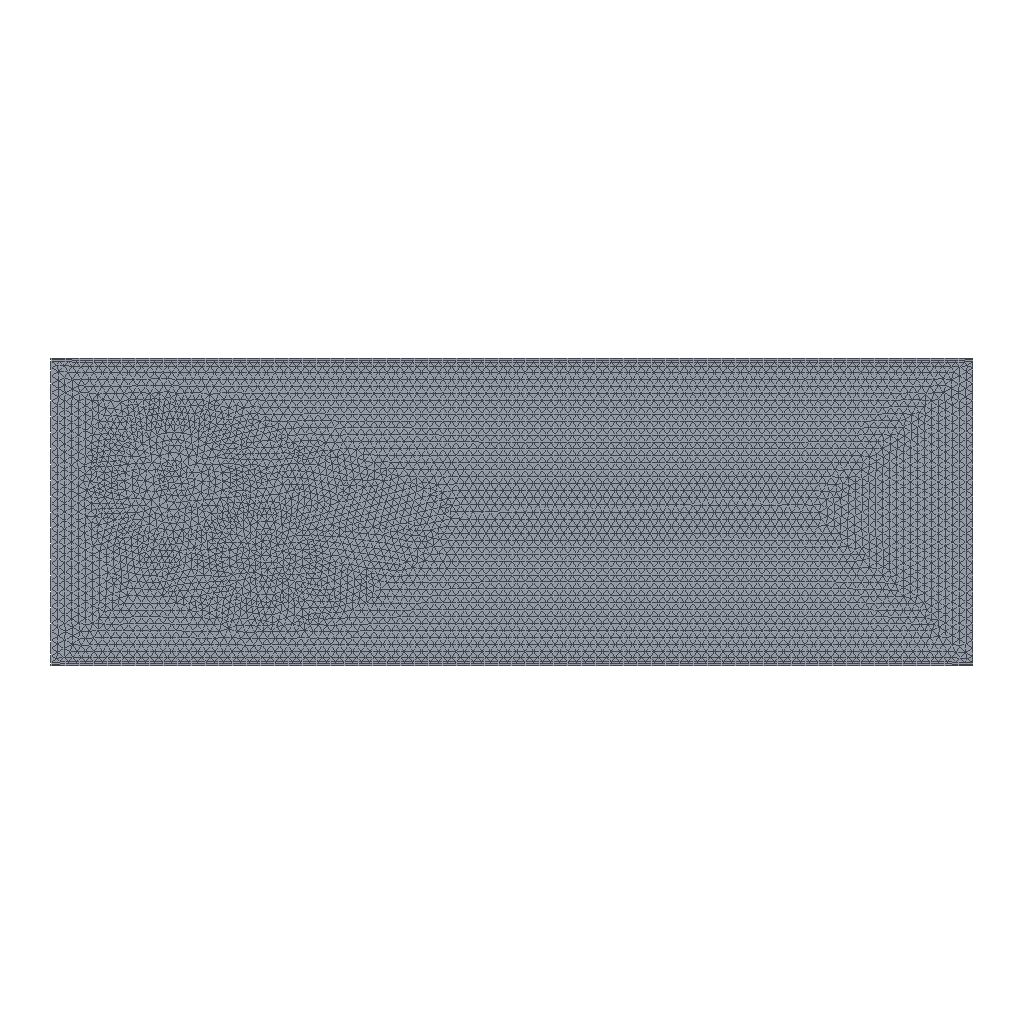Simulation study | comsol
Notes in the study folder:
rho_water 1e3[kg/m^3] Density, water
mu_water 1.002e-3[Pa*s] Dynamic viscosity, water
perm_water 8.0e1[1] Permittivity, water
rho_oil 8.84e2[kg/m^3] Density, oil
mu_oil 4.74e-1[Pa*s] Dynamic viscosity, oil
perm_oil 2.2[1] Permittivity, oil
Notes in the study folder:
epsilon_r tpf.Vf1*perm_water+tpf.Vf2*perm_oil Phase dependent permittivity
Tem11 -epsilon0_const*epsilon_r/2*(es.Ex^2+es.Ey^2)+epsilon0_const*epsilon_r*es.Ex^2 Maxwell stress tensor, 11-component
Tem22 -epsilon0_const*epsilon_r/2*(es.Ex^2+es.Ey^2)+epsilon0_const*epsilon_r*es.Ey^2 Maxwell stress tensor, 22-component
Tem12 epsilon0_const*epsilon_r*es.Ex*es.Ey Maxwell stress tensor, 12-component
Tem21 epsilon0_const*epsilon_r*es.Ex*es.Ey Maxwell stress tensor, 21-component
Fx d(Tem11,x)+d(Tem12,y) Force, x-component
Fy d(Tem21,x)+d(Tem22,y) Force, y-component
Set-up summary:
category,name,step,type,value,unit,region
solver,comsol,,COMSOL Multiphysics 6.4 (Build: 293)
units,SI; geometry length unit mm,,stated,COMSOL default unit system (SI)
analysis,Study 1,,TransientInitialization + Transient,space_dimension=2D
load_step,std1/transi,std1/transi,TransientInitialization + Transient,type=TransientInitialization; times=0..1 (11 values)
load_step,std1/time,std1/time,TransientInitialization + Transient,"type=Transient; times=range(0,0.05,0.3)"
mesh,nodes,,,5746
mesh,elements,,,10768
element_type,tri,,,10340
element_type,quad,,,428
element_type,edg,,,358
element_type,vtx,,,12
component,mod1,,2D,geometry=geom1; domains=3
physics,Electrostatics (es),mod1,Electrostatics,"V(V), D(Dx Dy Dz)"
physics,"Laminar Two-Phase Flow, Phase Field (tpf)",mod1,LaminarTwoPhaseFlowPhaseField,"u(u v w), p(p), phils(phils), phipf(phipf), psi(psi), k(k), ep(ep), GI(GI)"
parameter,rho_water,,,1e3[kg/m^3]
parameter,mu_water,,,1.002e-3[Pa*s]
parameter,perm_water,,,8.0e1[1]
parameter,rho_oil,,,8.84e2[kg/m^3]
parameter,mu_oil,,,4.74e-1[Pa*s]
parameter,perm_oil,,,2.2[1]
material,Water,,relpermittivity,perm_water,,selection []
material,Water,,density,rho_water,,selection []
material,Water,,dynamicviscosity,mu_water,,selection []
material,Oil,,relpermittivity,perm_oil,,"selection [2, 3]"
material,Oil,,density,rho_oil,,"selection [2, 3]"
material,Oil,,dynamicviscosity,mu_oil,,"selection [2, 3]"
bc,Charge Conservation 1 (ccn1),mod1/es,ChargeConservationSolid,epsilonr=epsilon_r; epsilonBis=0; epsilonPrim=1; P=0 0 0; Dr=0 0 0; ConstitutiveRelationDE=RelativePermittivity; materialType=solid; AllowSolidMaterials=1; epsilonrS=1; PolarizationModel=LangevinFunction; Lfunction=es.normEeff/(es.normEeff+(2.49e6[m/F]*es.Psat)) es.normEeff/(es.normEeff+(2.5e6[m/F]*es.Psat)) 0; EffectiveField=useTotal; Eeff=es.Emgx es.Emgy es.Emgz; Hysteresis=0; DR=0 0 0; Psat=0.4,,"selection [1, 2, 3]"
bc,Zero Charge 1 (zc1),mod1/es,ZeroCharge,,,"selection [1, 4]"
bc,Initial Values 1 (init1),mod1/es,init,V=0; D=0 0 0,,"selection [1, 2, 3]"
bc,Electric Potential 1 (pot1),mod1/es,ElectricPotential,V0=5e3[V],,selection [3]
bc,Electric Potential 2 (pot2),mod1/es,ElectricPotential,V0=0[V],,selection [2]
bc,Fluid Properties 1 (fp1),mod1/tpf,FluidProperties,rho1=0; mu1=0; rho2=0; mu2=0; sigma=3.1e-2[N/m]; NeglectSurfaceTension=0; SurfaceTensionCoefficient=userdef; LibraryCoefficientLiquidGas=WaterAir; LibraryCoefficientLiquidLiquid=BenzeneWater20; epsilon_ls=tpf.hmax/2; gamma=1; dfdphi=0; epsilon_pf=tpf.hmax/2; chi=1; Fluid1=mat1; Fluid2=mat2; mu01=1e-3[Pa*s]; mu_inf1=0; n_car1=0; lam_car1=0; mu02=1e-3[Pa*s]; mu_inf2=0; n_car2=0; lam_car2=0; m_pow1=1,,"selection [1, 2, 3]"
bc,Wall 1 (wall1),mod1/tpf,Wall,T=293.15[K]; E=0 0 0; BoundaryCondition=NoSlip; uwall=0 0 0; ElectroosmoticOption=userdef; zeta=-0.1[V]; mueo=7e-8[m^2/(V*s)]; UseViscousSlip=0; UseThermalCreep=0; SlipLengthOption=userdef; Ls=1e-7[m]; alphav=0.9; sigmat=0.75; epsilonr=80; lambda=1e-6[m]; uvw=0; vw=0; uvwwall=0 0 0; uleak=0 0 0; thetaw=pi/2; beta=h; weakConstraints=0; ApplyWallRoughness=0; RoughnessModel=SandRoughness; ks=3.2[um];,,"selection [2, 3]"
bc,Initial Values 1 (init1),mod1/tpf,init,u=0 0 0; p=0; k=tpf.kinit; ep=tpf.epinit; FluidInitiallyInDomain=Fluid1phipf; GI=tpf.G0i; phipf=0; phils=0,,"selection [2, 3]"
bc,Flow continuity (dcont1),mod1/tpf,ContinuityFlow,pairDisconnect=1; pairSelection=all; pairsList=0,,selection []
bc,Initial Values 2 (init2),mod1/tpf,init,u=0 0 0; p=0; k=tpf.kinit; ep=tpf.epinit; FluidInitiallyInDomain=Fluid2phipf; GI=tpf.G0i; phipf=0; phils=0,,selection [1]
bc,Volume Force 1 (vf1),mod1/tpf,VolumeForce,F=Fx Fy 0,,"selection [1, 2, 3]"
bc,Inlet 1 (inl1),mod1/tpf,Inlet,weakConstraints=0; BoundaryCondition=Velocity; ComponentWise=NormalInflowVelocity; p0=0; f0=0; U0in=50[mm/s]; u0=0 0 0; LaminarInflowOption=Uav; Uav=0; V0=0; Lentr=1; p0_entr=0; ConstrainEndPointsToZero=0; Dzentr=1; RANSVarOption=SpecifyTurbulentLengthScaleAndIntensity; IT=0.05; LT=0.01; k0=0.005; ep0=0.005; Uref=1; phi0=0; Vf0=1; Mn=0.032[kg/mol]; Mf=0; Pst=1[atm]; Tst=273.15[K]; mnst=0.02241[m,,selection [1]
bc,Outlet 1 (out1),mod1/tpf,Outlet,weakConstraints=0; BoundaryCondition=PressureNoViscousStress; ComponentWise=NormalOutflowVelocity; p0=0; U0out=0; u0=0 0 0; f0=0; LaminarOutflowOption=Uav; Uav=0; V0=0; Lexit=1; p0_exit=0; ConstrainEndPointsToZero=0; Dzexit=1,,selection [4]
bc,Initial Interface 1 (ii1),mod1/tpf,InitialInterface,,,"selection [5, 6, 7, 8, 9, 10, 11, 12]"
COMSOL model file for Java, long lists of numbers shortened:
/*
 * em_deck.java
 */

import com.comsol.model.*;
import com.comsol.model.util.*;

/** Model exported on Oct 28 2026, 10:34 by COMSOL 6.4.0.293. */
public class em_deck {

  public static Model run() {
    Model model = ModelUtil.create("Model");

    model.modelPath("");

    model.label("in.mph");

    model.param().set("rho_water", "1e3[kg/m^3]", "Density, water");
    model.param().set("mu_water", "1.002e-3[Pa*s]", "Dynamic viscosity, water");
    model.param().set("perm_water", "8.0e1[1]", "Permittivity, water");
    model.param().set("rho_oil", "8.84e2[kg/m^3]", "Density, oil");
    model.param().set("mu_oil", "4.74e-1[Pa*s]", "Dynamic viscosity, oil");
    model.param().set("perm_oil", "2.2[1]", "Permittivity, oil");

    model.component().create("mod1", false);

    model.component("mod1").geom().create("geom1", 2);

    model.component("mod1").label("Model 1");

    model.component("mod1").defineLocalCoord(false);

    model.component("mod1").curvedInterior(false);

    model.component("mod1").mesh().create("mesh1");

    model.component("mod1").geom("geom1").lengthUnit("mm");
    model.component("mod1").geom("geom1").repairTolType("relative");
    model.component("mod1").geom("geom1").create("r1", "Rectangle");
    model.component("mod1").geom("geom1").feature("r1").set("size", new String[]{"30[mm]", "10[mm]"});
    model.component("mod1").geom("geom1").create("c1", "Circle");
    model.component("mod1").geom("geom1").feature("c1").set("r", "1.6[mm]");
    model.component("mod1").geom("geom1").feature("c1").set("pos", new String[]{"4[mm]", "6[mm]"});
    model.component("mod1").geom("geom1").create("c2", "Circle");
    model.component("mod1").geom("geom1").feature("c2").set("r", "1.2[mm]");
    model.component("mod1").geom("geom1").feature("c2").set("pos", new String[]{"7[mm]", "3.5[mm]"});
    model.component("mod1").geom("geom1").feature("fin").set("repairtoltype", "relative");
    model.component("mod1").geom("geom1").run();

    model.component("mod1").selection().create("sel1", "Explicit");
    model.component("mod1").selection("sel1").geom("geom1", 1);
    model.component("mod1").selection("sel1").set(4);
    model.component("mod1").selection().create("sel2", "Explicit");
    model.component("mod1").selection("sel2").geom("geom1", 1);
    model.component("mod1").selection("sel2").set(1);
    model.component("mod1").selection().create("sel3", "Explicit");
    model.component("mod1").selection("sel3").geom("geom1", 1);
    model.component("mod1").selection("sel3").set(5, 6, 7, 8, 9, 10, 11, 12);
    model.component("mod1").selection("sel1").label("Outlet");
    model.component("mod1").selection("sel2").label("Inlet");
    model.component("mod1").selection("sel3").label("Oil/Water Interface");

    model.component("mod1").variable().create("var1");
    model.component("mod1").variable("var1")
         .set("epsilon_r", "tpf.Vf1*perm_water+tpf.Vf2*perm_oil", "Phase dependent permittivity");
    model.component("mod1").variable("var1")
         .set("Tem11", "-epsilon0_const*epsilon_r/2*(es.Ex^2+es.Ey^2)+epsilon0_const*epsilon_r*es.Ex^2", "Maxwell stress tensor, 11-component");
    model.component("mod1").variable("var1")
         .set("Tem22", "-epsilon0_const*epsilon_r/2*(es.Ex^2+es.Ey^2)+epsilon0_const*epsilon_r*es.Ey^2", "Maxwell stress tensor, 22-component");
    model.component("mod1").variable("var1")
         .set("Tem12", "epsilon0_const*epsilon_r*es.Ex*es.Ey", "Maxwell stress tensor, 12-component");
    model.component("mod1").variable("var1")
         .set("Tem21", "epsilon0_const*epsilon_r*es.Ex*es.Ey", "Maxwell stress tensor, 21-component");
    model.component("mod1").variable("var1").set("Fx", "d(Tem11,x)+d(Tem12,y)", "Force, x-component");
    model.component("mod1").variable("var1").set("Fy", "d(Tem21,x)+d(Tem22,y)", "Force, y-component");

    model.component("mod1").material().create("mat1", "Common");
    model.component("mod1").material().create("mat2", "Common");
    model.component("mod1").material("mat1").selection().set(2, 3);
    model.component("mod1").material("mat2").selection().set(2, 3);

    model.component("mod1").physics().create("es", "Electrostatics", "geom1");
    model.component("mod1").physics("es").create("ccn1", "ChargeConservationSolid", 2);
    model.component("mod1").physics("es").feature("ccn1").selection().all();
    model.component("mod1").physics("es").feature("ccn1").featureInfo().create("information");
    model.component("mod1").physics("es").create("pot1", "ElectricPotential", 1);
    model.component("mod1").physics("es").feature("pot1").selection().set(3);
    model.component("mod1").physics("es").create("pot2", "ElectricPotential", 1);
    model.component("mod1").physics("es").feature("pot2").selection().set(2);
    model.component("mod1").physics().create("tpf", "_Coded_LaminarTwoPhaseFlowPhaseField", "geom1");
    model.component("mod1").physics("tpf").create("dcont1", "ContinuityFlow", 1);
    model.component("mod1").physics("tpf").create("init2", "init", 2);
    model.component("mod1").physics("tpf").feature("init2").selection().set(1);
    model.component("mod1").physics("tpf").create("vf1", "VolumeForce", 2);
    model.component("mod1").physics("tpf").feature("vf1").selection().all();
    model.component("mod1").physics("tpf").create("inl1", "Inlet", 1);
    model.component("mod1").physics("tpf").feature("inl1").selection().named("sel2");
    model.component("mod1").physics("tpf").create("out1", "Outlet", 1);
    model.component("mod1").physics("tpf").feature("out1").selection().named("sel1");
    model.component("mod1").physics("tpf").create("ii1", "InitialInterface", 1);
    model.component("mod1").physics("tpf").feature("ii1").selection().named("sel3");

    model.component("mod1").mesh("mesh1").autoMeshSize(4);

    model.thermodynamics().label("Thermodynamics Package");

    model.component("mod1").view("view1").set("showlabels", true);
    model.component("mod1").view("view1").axis().set("xmin", -1.5);
    model.component("mod1").view("view1").axis().set("xmax", 31.5);
    model.component("mod1").view("view1").axis().set("ymin", -54.4);
    model.component("mod1").view("view1").axis().set("ymax", 64.4);

    model.component("mod1").material("mat1").label("Water");
    model.component("mod1").material("mat1").propertyGroup("def")
         .set("relpermittivity", new String[]{"perm_water", "0", "0", "0", "perm_water", "0", "0", "0", "perm_water"});
    model.component("mod1").material("mat1").propertyGroup("def").set("density", "rho_water");
    model.component("mod1").material("mat1").propertyGroup("def").set("dynamicviscosity", "mu_water");
    model.component("mod1").material("mat2").label("Oil");
    model.component("mod1").material("mat2").propertyGroup("def")
         .set("relpermittivity", new String[]{"perm_oil", "0", "0", "0", "perm_oil", "0", "0", "0", "perm_oil"});
    model.component("mod1").material("mat2").propertyGroup("def").set("density", "rho_oil");
    model.component("mod1").material("mat2").propertyGroup("def").set("dynamicviscosity", "mu_oil");

    model.component("mod1").physics("es").prop("ShapeProperty").set("order_electricpotential", 1);
    model.component("mod1").physics("es").prop("PortSweepSettings").set("PortParamName", "PortName");
    model.component("mod1").physics("es").feature("ccn1").set("epsilonr_mat", "userdef");
    model.component("mod1").physics("es").feature("ccn1")
         .set("epsilonr", new String[][]{{"epsilon_r"}, {"0"}, {"0"}, {"0"}, {"epsilon_r"}, {"0"}, {"0"}, {"0"}, {"epsilon_r"}});
    model.component("mod1").physics("es").feature("ccn1")
         .set("epsilonBis", new int[][]{{0}, {0}, {0}, {0}, {0}, {0}, {0}, {0}, {0}});
    model.component("mod1").physics("es").feature("ccn1").set("minput_temperature_src", "userdef");
    model.component("mod1").physics("es").feature("ccn1").set("minput_electricfield_src", "root.mod1.es.Ex");
    model.component("mod1").physics("es").feature("ccn1").label("Charge Conservation 1");
    model.component("mod1").physics("es").feature("ccn1").featureInfo("information").label("Migrated Feature");
    model.component("mod1").physics("es").feature("pot1").set("V0", "5e3[V]");
    model.component("mod1").physics("es").feature("pot2").set("V0", "0[V]");
    model.component("mod1").physics("tpf").label("Laminar Two-Phase Flow, Phase Field");
    model.component("mod1").physics("tpf").prop("Stabilization").set("StreamlineDiffusion", false);
    model.component("mod1").physics("tpf").prop("Stabilization").set("CrosswindDiffusion", false);
    model.component("mod1").physics("tpf").prop("LevelSetStabilization").set("CrosswindDiffusionOldFormS", true);
    model.component("mod1").physics("tpf").prop("TurbulenceProperty").set("kappav", 0.42);
    model.component("mod1").physics("tpf").prop("TurbulenceProperty").set("sigmaw", 0.1);
    model.component("mod1").physics("tpf").prop("RANSStabilization").set("CrosswindDiffusionOldFormRANS", true);
    model.component("mod1").physics("tpf").feature("fp1").set("sigma", "3.1e-2[N/m]");
    model.component("mod1").physics("tpf").feature("fp1").set("SurfaceTensionCoefficient", "userdef");
    model.component("mod1").physics("tpf").feature("fp1").set("Fluid1", "mat1");
    model.component("mod1").physics("tpf").feature("fp1").set("Fluid2", "mat2");
    model.component("mod1").physics("tpf").feature("fp1").set("minput_velocity_src", "root.mod1.u");
    model.component("mod1").physics("tpf").feature("fp1").set("minput_strainreferencetemperature", 0);
    model.component("mod1").physics("tpf").feature("fp1").set("editModelInputs", true);
    model.component("mod1").physics("tpf").feature("wall1").set("constraintType", "symmetricConstraint");
    model.component("mod1").physics("tpf").feature("dcont1").set("pairDisconnect", true);
    model.component("mod1").physics("tpf").feature("dcont1").set("pairSelection", "all");
    model.component("mod1").physics("tpf").feature("dcont1").active(false);
    model.component("mod1").physics("tpf").feature("dcont1").label("Flow continuity");
    model.component("mod1").physics("tpf").feature("init2").set("FluidInitiallyInDomain", "Fluid2phipf");
    model.component("mod1").physics("tpf").feature("vf1").set("F", new String[][]{{"Fx"}, {"Fy"}, {"0"}});
    model.component("mod1").physics("tpf").feature("inl1").set("U0in", "50[mm/s]");
    model.component("mod1").physics("tpf").feature("inl1").set("LT", 0.01);
    model.component("mod1").physics("tpf").feature("inl1").set("k0", 0.005);
    model.component("mod1").physics("tpf").feature("inl1").set("ep0", 0.005);
    model.component("mod1").physics("tpf").feature("inl1").set("Uref", 1);
    model.component("mod1").physics("tpf").feature("inl1").set("Vf0", 1);

    model.study().create("std1");
    model.study("std1").create("transi", "TransientInitialization");
    model.study("std1").create("time", "Transient");

    model.sol().create("sol1");
    model.sol("sol1").attach("std1");
    model.sol("sol1").create("st1", "StudyStep");
    model.sol("sol1").create("v1", "Variables");
    model.sol("sol1").create("t1", "Time");
    model.sol("sol1").create("st2", "StudyStep");
    model.sol("sol1").create("v2", "Variables");
    model.sol("sol1").create("t2", "Time");
    model.sol("sol1").feature("t1").create("fc1", "FullyCoupled");
    model.sol("sol1").feature("t1").create("d1", "Direct");
    model.sol("sol1").feature("t1").feature().remove("fcDef");
    model.sol("sol1").feature("t2").create("fc1", "FullyCoupled");
    model.sol("sol1").feature("t2").create("d1", "Direct");
    model.sol("sol1").feature("t2").feature().remove("fcDef");

    model.result().create("pg1", "PlotGroup2D");
    model.result("pg1").create("surf1", "Surface");

    model.study("std1").feature("time").set("tlist", "range(0,0.05,0.3)");

    model.sol("sol1").label("Solver 1");
    model.sol("sol1").feature("st1").label("Compile Equations: Transient Initialization");
    model.sol("sol1").feature("v1").label("Dependent Variables 1.1");
    model.sol("sol1").feature("v1").set("clistctrl", new String[]{});
    model.sol("sol1").feature("v1").set("cname", new String[]{});
    model.sol("sol1").feature("v1").set("clist", new int[]{});
    model.sol("sol1").feature("t1").label("Time-Dependent Solver 1.1");
    model.sol("sol1").feature("t1").set("atolglobalmethod", "unscaled");
    model.sol("sol1").feature("t1").set("atolglobalvaluemethod", "manual");
    model.sol("sol1").feature("t1").set("atolglobal", "0.001");
    model.sol("sol1").feature("t1").set("ewtrescale", false);
    model.sol("sol1").feature("t1")
         .set("atolvaluemethod", new String[]{"mod1_V", "manual", "mod1_u", "manual", "mod1_psi", "manual", "mod1_p", "manual", "mod1_phipf", "manual",
         "mod1_GI", "factor"});
    model.sol("sol1").feature("t1").set("initialstepbdf", "0.001");
    model.sol("sol1").feature("t1").set("maxorder", 2);
    model.sol("sol1").feature("t1").set("bwinitstepfrac", "1.0");
    model.sol("sol1").feature("t1").set("estrat", "exclude");
    model.sol("sol1").feature("t1").feature("dDef").label("Direct 2");
    model.sol("sol1").feature("t1").feature("dDef").set("thresh", 0.1);
    model.sol("sol1").feature("t1").feature("dDef").set("ooc", false);
    model.sol("sol1").feature("t1").feature("dDef").set("rhob", 400);
    model.sol("sol1").feature("t1").feature("aDef").label("Advanced 1");
    model.sol("sol1").feature("t1").feature("fc1").label("Fully Coupled 1.1");
    model.sol("sol1").feature("t1").feature("fc1").set("maxiter", 5);
    model.sol("sol1").feature("t1").feature("fc1").set("jtech", "once");
    model.sol("sol1").feature("t1").feature("fc1").set("probesel", "manual");
    model.sol("sol1").feature("t1").feature("d1").label("Direct 1.1");
    model.sol("sol1").feature("t1").feature("d1").set("linsolver", "pardiso");
    model.sol("sol1").feature("t1").feature("d1").set("ooc", false);
    model.sol("sol1").feature("t1").feature("d1").set("pardreorder", "ndmt");
    model.sol("sol1").feature("t1").feature("d1").set("pivotstrategy", false);
    model.sol("sol1").feature("t1").feature("d1").set("rhob", 400);
    model.sol("sol1").feature("st2").label("Compile Equations: Time Dependent (2)");
    model.sol("sol1").feature("st2").set("studystep", "time");
    model.sol("sol1").feature("v2").label("Dependent Variables 2.1");
    model.sol("sol1").feature("v2").set("initmethod", "sol");
    model.sol("sol1").feature("v2").set("initsol", "sol1");
    model.sol("sol1").feature("v2").set("solnum", "auto");
    model.sol("sol1").feature("v2").set("scalemethod", "manual");
    model.sol("sol1").feature("v2").set("notsolmethod", "sol");
    model.sol("sol1").feature("v2").set("notsol", "sol1");
    model.sol("sol1").feature("v2").set("notsolnum", "auto");
    model.sol("sol1").feature("v2").set("clistctrl", new String[]{});
    model.sol("sol1").feature("v2").set("cname", new String[]{});
    model.sol("sol1").feature("v2").set("clist", new int[]{});
    model.sol("sol1").feature("v2").feature("mod1_V").set("scalemethod", "manual");
    model.sol("sol1").feature("v2").feature("mod1_V").set("scaleval", "1e3");
    model.sol("sol1").feature("v2").feature("mod1_u").set("scalemethod", "manual");
    model.sol("sol1").feature("v2").feature("mod1_u").set("scaleval", 0.1);
    model.sol("sol1").feature("v2").feature("mod1_psi").set("scalemethod", "manual");
    model.sol("sol1").feature("v2").feature("mod1_psi").set("scaleval", 0.1);
    model.sol("sol1").feature("v2").feature("mod1_p").set("scalemethod", "manual");
    model.sol("sol1").feature("v2").feature("mod1_p").set("scaleval", "1e3");
    model.sol("sol1").feature("t2").label("Time-Dependent Solver 2.1");
    model.sol("sol1").feature("t2").set("tlist", "range(0,0.05,0.3)");
    model.sol("sol1").feature("t2").set("atolglobalvaluemethod", "manual");
    model.sol("sol1").feature("t2").set("atolglobal", "0.001");
    model.sol("sol1").feature("t2").set("ewtrescale", false);
    model.sol("sol1").feature("t2")
         .set("atolvaluemethod", new String[]{"mod1_V", "manual", "mod1_u", "manual", "mod1_psi", "manual", "mod1_p", "manual", "mod1_phipf", "manual",
         "mod1_GI", "factor"});
    model.sol("sol1").feature("t2").set("initialstepbdf", "0.001");
    model.sol("sol1").feature("t2").set("maxorder", 2);
    model.sol("sol1").feature("t2").set("bwinitstepfrac", "1.0");
    model.sol("sol1").feature("t2").set("estrat", "exclude");
    model.sol("sol1").feature("t2").feature("dDef").label("Direct 2");
    model.sol("sol1").feature("t2").feature("dDef").set("thresh", 0.1);
    model.sol("sol1").feature("t2").feature("dDef").set("ooc", false);
    model.sol("sol1").feature("t2").feature("dDef").set("rhob", 400);
    model.sol("sol1").feature("t2").feature("aDef").label("Advanced 1");
    model.sol("sol1").feature("t2").feature("fc1").label("Fully Coupled 1.1");
    model.sol("sol1").feature("t2").feature("fc1").set("maxiter", 5);
    model.sol("sol1").feature("t2").feature("fc1").set("jtech", "once");
    model.sol("sol1").feature("t2").feature("fc1").set("probesel", "manual");
    model.sol("sol1").feature("t2").feature("d1").label("Direct 1.1");
    model.sol("sol1").feature("t2").feature("d1").set("thresh", 0.1);
    model.sol("sol1").feature("t2").feature("d1").set("ooc", false);
    model.sol("sol1").feature("t2").feature("d1").set("rhob", 400);

    model.study("std1").runNoGen();

    model.result().dataset("dset1").label("Solution 1");
    model.result().dataset("dset1").set("frametype", "material");
    model.result("pg1").set("smooth", "internal");
    model.result("pg1").feature("surf1").set("colortable", "RainbowClassic");
    model.result("pg1").feature("surf1").set("smooth", "internal");
    model.result("pg1").feature("surf1").set("resolution", "normal");

    return model;
  }

  public static void main(String[] args) {
    run();
  }

}
Results summary:
result,max V = abs(mod1.V),dset1 (7 solution(s)),,5000,V
result,max u = sqrt(abs(mod1.u)^2+abs(mod1.v)^2),dset1 (7 solution(s)),,0.1044,m/s